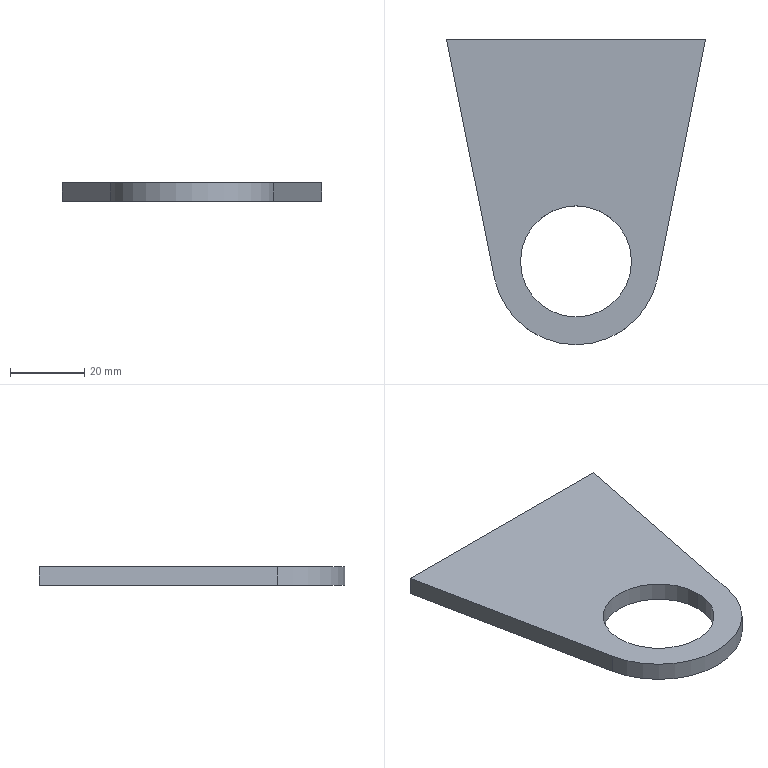Part | STEP file | Spring hanging buckle | 1 solid | 8 faces | box 70 x 82.5 x 5 mm | volume 17833 mm3 | plane 5 | cylinder 3 | commonest cylinder face diameters 30 x2 45 x1
STEP:
#1=CARTESIAN_POINT('',(0.,0.,0.));
#2=DIRECTION('',(0.,0.,1.));
#3=DIRECTION('',(1.,0.,0.));
#4=AXIS2_PLACEMENT_3D('',#1,#2,#3);
#5=CARTESIAN_POINT('',(-15.,0.,2.5));
#6=VERTEX_POINT('',#5);
#7=CARTESIAN_POINT('',(-15.,0.,-2.5));
#8=VERTEX_POINT('',#7);
#9=CARTESIAN_POINT('',(-15.,0.,2.5));
#10=DIRECTION('',(0.,0.,-1.));
#11=VECTOR('',#10,1.);
#12=LINE('',#9,#11);
#13=CARTESIAN_POINT('',(0.,0.,2.5));
#14=DIRECTION('',(0.,0.,-1.));
#15=DIRECTION('',(-1.,0.,0.));
#16=AXIS2_PLACEMENT_3D('',#13,#14,#15);
#17=CYLINDRICAL_SURFACE('',#16,15.);
#18=CARTESIAN_POINT('',(6.283,0.));
#19=DIRECTION('',(0.,1.));
#20=VECTOR('',#19,1.);
#21=LINE('',#18,#20);
#22=(GEOMETRIC_REPRESENTATION_CONTEXT(2)PARAMETRIC_REPRESENTATION_CONTEXT()REPRESENTATION_CONTEXT('',''));
#23=DEFINITIONAL_REPRESENTATION('',(#21),#22);
#24=PCURVE('',#17,#23);
#25=CARTESIAN_POINT('',(0.,0.,2.5));
#26=DIRECTION('',(0.,0.,-1.));
#27=DIRECTION('',(-1.,0.,0.));
#28=AXIS2_PLACEMENT_3D('',#25,#26,#27);
#29=CYLINDRICAL_SURFACE('',#28,15.);
#30=CARTESIAN_POINT('',(0.,0.));
#31=DIRECTION('',(0.,1.));
#32=VECTOR('',#31,1.);
#33=LINE('',#30,#32);
#34=(GEOMETRIC_REPRESENTATION_CONTEXT(2)PARAMETRIC_REPRESENTATION_CONTEXT()REPRESENTATION_CONTEXT('',''));
#35=DEFINITIONAL_REPRESENTATION('',(#33),#34);
#36=PCURVE('',#29,#35);
#37=SURFACE_CURVE('',#12,(#24,#36),.PCURVE_S1.);
#38=EDGE_CURVE('',#6,#8,#37,.T.);
#39=ORIENTED_EDGE('',*,*,#38,.T.);
#40=CARTESIAN_POINT('',(15.,0.,-2.5));
#41=VERTEX_POINT('',#40);
#42=CARTESIAN_POINT('',(0.,0.,-2.5));
#43=DIRECTION('',(0.,0.,1.));
#44=DIRECTION('',(-1.,0.,0.));
#45=AXIS2_PLACEMENT_3D('',#42,#43,#44);
#46=CIRCLE('',#45,15.);
#47=CARTESIAN_POINT('',(6.283,5.));
#48=DIRECTION('',(-1.,0.));
#49=VECTOR('',#48,1.);
#50=LINE('',#47,#49);
#51=(GEOMETRIC_REPRESENTATION_CONTEXT(2)PARAMETRIC_REPRESENTATION_CONTEXT()REPRESENTATION_CONTEXT('',''));
#52=DEFINITIONAL_REPRESENTATION('',(#50),#51);
#53=PCURVE('',#17,#52);
#54=CARTESIAN_POINT('',(0.,0.,-2.5));
#55=DIRECTION('',(0.,0.,1.));
#56=DIRECTION('',(1.,0.,0.));
#57=AXIS2_PLACEMENT_3D('',#54,#55,#56);
#58=PLANE('',#57);
#59=CARTESIAN_POINT('',(0.,0.));
#60=DIRECTION('',(-1.,0.));
#61=AXIS2_PLACEMENT_2D('',#59,#60);
#62=CIRCLE('',#61,15.);
#63=(GEOMETRIC_REPRESENTATION_CONTEXT(2)PARAMETRIC_REPRESENTATION_CONTEXT()REPRESENTATION_CONTEXT('',''));
#64=DEFINITIONAL_REPRESENTATION('',(#62),#63);
#65=PCURVE('',#58,#64);
#66=SURFACE_CURVE('',#46,(#53,#65),.PCURVE_S1.);
#67=EDGE_CURVE('',#8,#41,#66,.T.);
#68=ORIENTED_EDGE('',*,*,#67,.T.);
#69=CARTESIAN_POINT('',(15.,0.,2.5));
#70=VERTEX_POINT('',#69);
#71=CARTESIAN_POINT('',(15.,0.,2.5));
#72=DIRECTION('',(0.,0.,-1.));
#73=VECTOR('',#72,1.);
#74=LINE('',#71,#73);
#75=CARTESIAN_POINT('',(3.142,0.));
#76=DIRECTION('',(0.,1.));
#77=VECTOR('',#76,1.);
#78=LINE('',#75,#77);
#79=(GEOMETRIC_REPRESENTATION_CONTEXT(2)PARAMETRIC_REPRESENTATION_CONTEXT()REPRESENTATION_CONTEXT('',''));
#80=DEFINITIONAL_REPRESENTATION('',(#78),#79);
#81=PCURVE('',#17,#80);
#82=CARTESIAN_POINT('',(3.142,0.));
#83=DIRECTION('',(0.,1.));
#84=VECTOR('',#83,1.);
#85=LINE('',#82,#84);
#86=(GEOMETRIC_REPRESENTATION_CONTEXT(2)PARAMETRIC_REPRESENTATION_CONTEXT()REPRESENTATION_CONTEXT('',''));
#87=DEFINITIONAL_REPRESENTATION('',(#85),#86);
#88=PCURVE('',#29,#87);
#89=SURFACE_CURVE('',#74,(#81,#88),.PCURVE_S1.);
#90=EDGE_CURVE('',#70,#41,#89,.T.);
#91=ORIENTED_EDGE('',*,*,#90,.F.);
#92=CARTESIAN_POINT('',(0.,0.,2.5));
#93=DIRECTION('',(0.,0.,-1.));
#94=DIRECTION('',(-1.,0.,0.));
#95=AXIS2_PLACEMENT_3D('',#92,#93,#94);
#96=CIRCLE('',#95,15.);
#97=CARTESIAN_POINT('',(0.,0.));
#98=DIRECTION('',(1.,0.));
#99=VECTOR('',#98,1.);
#100=LINE('',#97,#99);
#101=(GEOMETRIC_REPRESENTATION_CONTEXT(2)PARAMETRIC_REPRESENTATION_CONTEXT()REPRESENTATION_CONTEXT('',''));
#102=DEFINITIONAL_REPRESENTATION('',(#100),#101);
#103=PCURVE('',#17,#102);
#104=CARTESIAN_POINT('',(0.,0.,2.5));
#105=DIRECTION('',(0.,0.,1.));
#106=DIRECTION('',(1.,0.,0.));
#107=AXIS2_PLACEMENT_3D('',#104,#105,#106);
#108=PLANE('',#107);
#109=CARTESIAN_POINT('',(-15.,0.));
#110=CARTESIAN_POINT('',(-15.,25.981));
#111=CARTESIAN_POINT('',(7.5,12.99));
#112=CARTESIAN_POINT('',(30.,0.));
#113=CARTESIAN_POINT('',(7.5,-12.99));
#114=CARTESIAN_POINT('',(-15.,-25.981));
#115=CARTESIAN_POINT('',(-15.,0.));
#116=(BOUNDED_CURVE()B_SPLINE_CURVE(2,(#109,#110,#111,#112,#113,#114,#115),.UNSPECIFIED.,.T.,.F.)B_SPLINE_CURVE_WITH_KNOTS((1,2,2,2,2,1),(-2.094,0.,2.094,4.189,6.283,8.378),.UNSPECIFIED.)CURVE()GEOMETRIC_REPRESENTATION_ITEM()RATIONAL_B_SPLINE_CURVE((1.,0.5,1.,0.5,1.,0.5,1.))REPRESENTATION_ITEM(''));
#117=(GEOMETRIC_REPRESENTATION_CONTEXT(2)PARAMETRIC_REPRESENTATION_CONTEXT()REPRESENTATION_CONTEXT('',''));
#118=DEFINITIONAL_REPRESENTATION('',(#116),#117);
#119=PCURVE('',#108,#118);
#120=SURFACE_CURVE('',#96,(#103,#119),.PCURVE_S1.);
#121=EDGE_CURVE('',#70,#6,#120,.T.);
#122=ORIENTED_EDGE('',*,*,#121,.T.);
#123=EDGE_LOOP('',(#39,#68,#91,#122));
#124=FACE_BOUND('',#123,.F.);
#125=ADVANCED_FACE('',(#124),#17,.F.);
#126=CARTESIAN_POINT('',(0.,0.,2.5));
#127=DIRECTION('',(0.,0.,-1.));
#128=DIRECTION('',(-1.,0.,0.));
#129=AXIS2_PLACEMENT_3D('',#126,#127,#128);
#130=CIRCLE('',#129,15.);
#131=CARTESIAN_POINT('',(-15.,0.));
#132=CARTESIAN_POINT('',(-15.,25.981));
#133=CARTESIAN_POINT('',(7.5,12.99));
#134=CARTESIAN_POINT('',(30.,0.));
#135=CARTESIAN_POINT('',(7.5,-12.99));
#136=CARTESIAN_POINT('',(-15.,-25.981));
#137=CARTESIAN_POINT('',(-15.,0.));
#138=(BOUNDED_CURVE()B_SPLINE_CURVE(2,(#131,#132,#133,#134,#135,#136,#137),.UNSPECIFIED.,.T.,.F.)B_SPLINE_CURVE_WITH_KNOTS((1,2,2,2,2,1),(-2.094,0.,2.094,4.189,6.283,8.378),.UNSPECIFIED.)CURVE()GEOMETRIC_REPRESENTATION_ITEM()RATIONAL_B_SPLINE_CURVE((1.,0.5,1.,0.5,1.,0.5,1.))REPRESENTATION_ITEM(''));
#139=(GEOMETRIC_REPRESENTATION_CONTEXT(2)PARAMETRIC_REPRESENTATION_CONTEXT()REPRESENTATION_CONTEXT('',''));
#140=DEFINITIONAL_REPRESENTATION('',(#138),#139);
#141=PCURVE('',#108,#140);
#142=CARTESIAN_POINT('',(0.,0.));
#143=DIRECTION('',(1.,0.));
#144=VECTOR('',#143,1.);
#145=LINE('',#142,#144);
#146=(GEOMETRIC_REPRESENTATION_CONTEXT(2)PARAMETRIC_REPRESENTATION_CONTEXT()REPRESENTATION_CONTEXT('',''));
#147=DEFINITIONAL_REPRESENTATION('',(#145),#146);
#148=PCURVE('',#29,#147);
#149=SURFACE_CURVE('',#130,(#141,#148),.PCURVE_S1.);
#150=EDGE_CURVE('',#6,#70,#149,.T.);
#151=ORIENTED_EDGE('',*,*,#150,.T.);
#152=ORIENTED_EDGE('',*,*,#121,.T.);
#153=EDGE_LOOP('',(#151,#152));
#154=FACE_BOUND('',#153,.T.);
#155=CARTESIAN_POINT('',(35.,60.,2.5));
#156=VERTEX_POINT('',#155);
#157=CARTESIAN_POINT('',(-35.,60.,2.5));
#158=VERTEX_POINT('',#157);
#159=CARTESIAN_POINT('',(0.,60.,2.5));
#160=DIRECTION('',(-1.,0.,0.));
#161=VECTOR('',#160,1.);
#162=LINE('',#159,#161);
#163=CARTESIAN_POINT('',(0.,60.));
#164=DIRECTION('',(-1.,0.));
#165=VECTOR('',#164,1.);
#166=LINE('',#163,#165);
#167=(GEOMETRIC_REPRESENTATION_CONTEXT(2)PARAMETRIC_REPRESENTATION_CONTEXT()REPRESENTATION_CONTEXT('',''));
#168=DEFINITIONAL_REPRESENTATION('',(#166),#167);
#169=PCURVE('',#108,#168);
#170=CARTESIAN_POINT('',(35.,60.,2.5));
#171=DIRECTION('',(0.,-1.,0.));
#172=DIRECTION('',(1.,0.,0.));
#173=AXIS2_PLACEMENT_3D('',#170,#171,#172);
#174=PLANE('',#173);
#175=CARTESIAN_POINT('',(-35.,0.));
#176=DIRECTION('',(-1.,0.));
#177=VECTOR('',#176,1.);
#178=LINE('',#175,#177);
#179=(GEOMETRIC_REPRESENTATION_CONTEXT(2)PARAMETRIC_REPRESENTATION_CONTEXT()REPRESENTATION_CONTEXT('',''));
#180=DEFINITIONAL_REPRESENTATION('',(#178),#179);
#181=PCURVE('',#174,#180);
#182=SURFACE_CURVE('',#162,(#169,#181),.PCURVE_S1.);
#183=EDGE_CURVE('',#156,#158,#182,.T.);
#184=ORIENTED_EDGE('',*,*,#183,.T.);
#185=CARTESIAN_POINT('',(-22.059,-4.431,2.5));
#186=VERTEX_POINT('',#185);
#187=CARTESIAN_POINT('',(-35.,60.,2.5));
#188=DIRECTION('',(0.1969,-0.9804,0.));
#189=VECTOR('',#188,1.);
#190=LINE('',#187,#189);
#191=CARTESIAN_POINT('',(-35.,60.));
#192=DIRECTION('',(0.1969,-0.9804));
#193=VECTOR('',#192,1.);
#194=LINE('',#191,#193);
#195=(GEOMETRIC_REPRESENTATION_CONTEXT(2)PARAMETRIC_REPRESENTATION_CONTEXT()REPRESENTATION_CONTEXT('',''));
#196=DEFINITIONAL_REPRESENTATION('',(#194),#195);
#197=PCURVE('',#108,#196);
#198=CARTESIAN_POINT('',(-35.,60.,2.5));
#199=DIRECTION('',(0.9804,0.1969,0.));
#200=DIRECTION('',(-0.1969,0.9804,0.));
#201=AXIS2_PLACEMENT_3D('',#198,#199,#200);
#202=PLANE('',#201);
#203=CARTESIAN_POINT('',(0.,0.));
#204=DIRECTION('',(-1.,0.));
#205=VECTOR('',#204,1.);
#206=LINE('',#203,#205);
#207=(GEOMETRIC_REPRESENTATION_CONTEXT(2)PARAMETRIC_REPRESENTATION_CONTEXT()REPRESENTATION_CONTEXT('',''));
#208=DEFINITIONAL_REPRESENTATION('',(#206),#207);
#209=PCURVE('',#202,#208);
#210=SURFACE_CURVE('',#190,(#197,#209),.PCURVE_S1.);
#211=EDGE_CURVE('',#158,#186,#210,.T.);
#212=ORIENTED_EDGE('',*,*,#211,.T.);
#213=CARTESIAN_POINT('',(22.059,-4.431,2.5));
#214=VERTEX_POINT('',#213);
#215=CARTESIAN_POINT('',(0.,0.,2.5));
#216=DIRECTION('',(0.,0.,1.));
#217=DIRECTION('',(-1.,0.,0.));
#218=AXIS2_PLACEMENT_3D('',#215,#216,#217);
#219=CIRCLE('',#218,22.5);
#220=CARTESIAN_POINT('',(0.,0.));
#221=DIRECTION('',(-1.,0.));
#222=AXIS2_PLACEMENT_2D('',#220,#221);
#223=CIRCLE('',#222,22.5);
#224=(GEOMETRIC_REPRESENTATION_CONTEXT(2)PARAMETRIC_REPRESENTATION_CONTEXT()REPRESENTATION_CONTEXT('',''));
#225=DEFINITIONAL_REPRESENTATION('',(#223),#224);
#226=PCURVE('',#108,#225);
#227=CARTESIAN_POINT('',(0.,0.,2.5));
#228=DIRECTION('',(0.,0.,-1.));
#229=DIRECTION('',(-1.,0.,0.));
#230=AXIS2_PLACEMENT_3D('',#227,#228,#229);
#231=CYLINDRICAL_SURFACE('',#230,22.5);
#232=CARTESIAN_POINT('',(6.283,0.));
#233=DIRECTION('',(-1.,0.));
#234=VECTOR('',#233,1.);
#235=LINE('',#232,#234);
#236=(GEOMETRIC_REPRESENTATION_CONTEXT(2)PARAMETRIC_REPRESENTATION_CONTEXT()REPRESENTATION_CONTEXT('',''));
#237=DEFINITIONAL_REPRESENTATION('',(#235),#236);
#238=PCURVE('',#231,#237);
#239=SURFACE_CURVE('',#219,(#226,#238),.PCURVE_S1.);
#240=EDGE_CURVE('',#186,#214,#239,.T.);
#241=ORIENTED_EDGE('',*,*,#240,.T.);
#242=CARTESIAN_POINT('',(22.059,-4.431,2.5));
#243=DIRECTION('',(0.1969,0.9804,0.));
#244=VECTOR('',#243,1.);
#245=LINE('',#242,#244);
#246=CARTESIAN_POINT('',(22.059,-4.431));
#247=DIRECTION('',(0.1969,0.9804));
#248=VECTOR('',#247,1.);
#249=LINE('',#246,#248);
#250=(GEOMETRIC_REPRESENTATION_CONTEXT(2)PARAMETRIC_REPRESENTATION_CONTEXT()REPRESENTATION_CONTEXT('',''));
#251=DEFINITIONAL_REPRESENTATION('',(#249),#250);
#252=PCURVE('',#108,#251);
#253=CARTESIAN_POINT('',(22.059,-4.431,2.5));
#254=DIRECTION('',(-0.9804,0.1969,0.));
#255=DIRECTION('',(-0.1969,-0.9804,0.));
#256=AXIS2_PLACEMENT_3D('',#253,#254,#255);
#257=PLANE('',#256);
#258=CARTESIAN_POINT('',(0.,0.));
#259=DIRECTION('',(-1.,0.));
#260=VECTOR('',#259,1.);
#261=LINE('',#258,#260);
#262=(GEOMETRIC_REPRESENTATION_CONTEXT(2)PARAMETRIC_REPRESENTATION_CONTEXT()REPRESENTATION_CONTEXT('',''));
#263=DEFINITIONAL_REPRESENTATION('',(#261),#262);
#264=PCURVE('',#257,#263);
#265=SURFACE_CURVE('',#245,(#252,#264),.PCURVE_S1.);
#266=EDGE_CURVE('',#214,#156,#265,.T.);
#267=ORIENTED_EDGE('',*,*,#266,.T.);
#268=EDGE_LOOP('',(#184,#212,#241,#267));
#269=FACE_BOUND('',#268,.T.);
#270=ADVANCED_FACE('',(#154,#269),#108,.T.);
#271=CARTESIAN_POINT('',(0.,0.,-2.5));
#272=DIRECTION('',(0.,0.,1.));
#273=DIRECTION('',(-1.,0.,0.));
#274=AXIS2_PLACEMENT_3D('',#271,#272,#273);
#275=CIRCLE('',#274,15.);
#276=CARTESIAN_POINT('',(6.283,5.));
#277=DIRECTION('',(-1.,0.));
#278=VECTOR('',#277,1.);
#279=LINE('',#276,#278);
#280=(GEOMETRIC_REPRESENTATION_CONTEXT(2)PARAMETRIC_REPRESENTATION_CONTEXT()REPRESENTATION_CONTEXT('',''));
#281=DEFINITIONAL_REPRESENTATION('',(#279),#280);
#282=PCURVE('',#29,#281);
#283=CARTESIAN_POINT('',(0.,0.));
#284=DIRECTION('',(-1.,0.));
#285=AXIS2_PLACEMENT_2D('',#283,#284);
#286=CIRCLE('',#285,15.);
#287=(GEOMETRIC_REPRESENTATION_CONTEXT(2)PARAMETRIC_REPRESENTATION_CONTEXT()REPRESENTATION_CONTEXT('',''));
#288=DEFINITIONAL_REPRESENTATION('',(#286),#287);
#289=PCURVE('',#58,#288);
#290=SURFACE_CURVE('',#275,(#282,#289),.PCURVE_S1.);
#291=EDGE_CURVE('',#41,#8,#290,.T.);
#292=ORIENTED_EDGE('',*,*,#291,.T.);
#293=ORIENTED_EDGE('',*,*,#38,.F.);
#294=ORIENTED_EDGE('',*,*,#150,.T.);
#295=ORIENTED_EDGE('',*,*,#90,.T.);
#296=EDGE_LOOP('',(#292,#293,#294,#295));
#297=FACE_BOUND('',#296,.F.);
#298=ADVANCED_FACE('',(#297),#29,.F.);
#299=CARTESIAN_POINT('',(-22.059,-4.431,-2.5));
#300=VERTEX_POINT('',#299);
#301=CARTESIAN_POINT('',(-22.059,-4.431,2.5));
#302=DIRECTION('',(0.,0.,-1.));
#303=VECTOR('',#302,1.);
#304=LINE('',#301,#303);
#305=CARTESIAN_POINT('',(-65.717,0.));
#306=DIRECTION('',(0.,-1.));
#307=VECTOR('',#306,1.);
#308=LINE('',#305,#307);
#309=(GEOMETRIC_REPRESENTATION_CONTEXT(2)PARAMETRIC_REPRESENTATION_CONTEXT()REPRESENTATION_CONTEXT('',''));
#310=DEFINITIONAL_REPRESENTATION('',(#308),#309);
#311=PCURVE('',#202,#310);
#312=CARTESIAN_POINT('',(6.085,0.));
#313=DIRECTION('',(0.,1.));
#314=VECTOR('',#313,1.);
#315=LINE('',#312,#314);
#316=(GEOMETRIC_REPRESENTATION_CONTEXT(2)PARAMETRIC_REPRESENTATION_CONTEXT()REPRESENTATION_CONTEXT('',''));
#317=DEFINITIONAL_REPRESENTATION('',(#315),#316);
#318=PCURVE('',#231,#317);
#319=SURFACE_CURVE('',#304,(#311,#318),.PCURVE_S1.);
#320=EDGE_CURVE('',#186,#300,#319,.T.);
#321=ORIENTED_EDGE('',*,*,#320,.F.);
#322=ORIENTED_EDGE('',*,*,#211,.F.);
#323=CARTESIAN_POINT('',(-35.,60.,-2.5));
#324=VERTEX_POINT('',#323);
#325=CARTESIAN_POINT('',(-35.,60.,2.5));
#326=DIRECTION('',(0.,0.,1.));
#327=VECTOR('',#326,1.);
#328=LINE('',#325,#327);
#329=CARTESIAN_POINT('',(0.,0.));
#330=DIRECTION('',(0.,1.));
#331=VECTOR('',#330,1.);
#332=LINE('',#329,#331);
#333=(GEOMETRIC_REPRESENTATION_CONTEXT(2)PARAMETRIC_REPRESENTATION_CONTEXT()REPRESENTATION_CONTEXT('',''));
#334=DEFINITIONAL_REPRESENTATION('',(#332),#333);
#335=PCURVE('',#202,#334);
#336=CARTESIAN_POINT('',(-70.,0.));
#337=DIRECTION('',(0.,1.));
#338=VECTOR('',#337,1.);
#339=LINE('',#336,#338);
#340=(GEOMETRIC_REPRESENTATION_CONTEXT(2)PARAMETRIC_REPRESENTATION_CONTEXT()REPRESENTATION_CONTEXT('',''));
#341=DEFINITIONAL_REPRESENTATION('',(#339),#340);
#342=PCURVE('',#174,#341);
#343=SURFACE_CURVE('',#328,(#335,#342),.PCURVE_S1.);
#344=EDGE_CURVE('',#324,#158,#343,.T.);
#345=ORIENTED_EDGE('',*,*,#344,.F.);
#346=CARTESIAN_POINT('',(-35.,60.,-2.5));
#347=DIRECTION('',(-0.1969,0.9804,0.));
#348=VECTOR('',#347,1.);
#349=LINE('',#346,#348);
#350=CARTESIAN_POINT('',(0.,-5.));
#351=DIRECTION('',(1.,0.));
#352=VECTOR('',#351,1.);
#353=LINE('',#350,#352);
#354=(GEOMETRIC_REPRESENTATION_CONTEXT(2)PARAMETRIC_REPRESENTATION_CONTEXT()REPRESENTATION_CONTEXT('',''));
#355=DEFINITIONAL_REPRESENTATION('',(#353),#354);
#356=PCURVE('',#202,#355);
#357=CARTESIAN_POINT('',(-35.,60.));
#358=DIRECTION('',(-0.1969,0.9804));
#359=VECTOR('',#358,1.);
#360=LINE('',#357,#359);
#361=(GEOMETRIC_REPRESENTATION_CONTEXT(2)PARAMETRIC_REPRESENTATION_CONTEXT()REPRESENTATION_CONTEXT('',''));
#362=DEFINITIONAL_REPRESENTATION('',(#360),#361);
#363=PCURVE('',#58,#362);
#364=SURFACE_CURVE('',#349,(#356,#363),.PCURVE_S1.);
#365=EDGE_CURVE('',#300,#324,#364,.T.);
#366=ORIENTED_EDGE('',*,*,#365,.F.);
#367=EDGE_LOOP('',(#321,#322,#345,#366));
#368=FACE_BOUND('',#367,.T.);
#369=ADVANCED_FACE('',(#368),#202,.F.);
#370=ORIENTED_EDGE('',*,*,#344,.T.);
#371=ORIENTED_EDGE('',*,*,#183,.F.);
#372=CARTESIAN_POINT('',(35.,60.,-2.5));
#373=VERTEX_POINT('',#372);
#374=CARTESIAN_POINT('',(35.,60.,2.5));
#375=DIRECTION('',(0.,0.,1.));
#376=VECTOR('',#375,1.);
#377=LINE('',#374,#376);
#378=CARTESIAN_POINT('',(0.,0.));
#379=DIRECTION('',(0.,1.));
#380=VECTOR('',#379,1.);
#381=LINE('',#378,#380);
#382=(GEOMETRIC_REPRESENTATION_CONTEXT(2)PARAMETRIC_REPRESENTATION_CONTEXT()REPRESENTATION_CONTEXT('',''));
#383=DEFINITIONAL_REPRESENTATION('',(#381),#382);
#384=PCURVE('',#174,#383);
#385=CARTESIAN_POINT('',(-65.717,0.));
#386=DIRECTION('',(0.,1.));
#387=VECTOR('',#386,1.);
#388=LINE('',#385,#387);
#389=(GEOMETRIC_REPRESENTATION_CONTEXT(2)PARAMETRIC_REPRESENTATION_CONTEXT()REPRESENTATION_CONTEXT('',''));
#390=DEFINITIONAL_REPRESENTATION('',(#388),#389);
#391=PCURVE('',#257,#390);
#392=SURFACE_CURVE('',#377,(#384,#391),.PCURVE_S1.);
#393=EDGE_CURVE('',#373,#156,#392,.T.);
#394=ORIENTED_EDGE('',*,*,#393,.F.);
#395=CARTESIAN_POINT('',(35.,60.,-2.5));
#396=DIRECTION('',(1.,0.,0.));
#397=VECTOR('',#396,1.);
#398=LINE('',#395,#397);
#399=CARTESIAN_POINT('',(0.,-5.));
#400=DIRECTION('',(1.,0.));
#401=VECTOR('',#400,1.);
#402=LINE('',#399,#401);
#403=(GEOMETRIC_REPRESENTATION_CONTEXT(2)PARAMETRIC_REPRESENTATION_CONTEXT()REPRESENTATION_CONTEXT('',''));
#404=DEFINITIONAL_REPRESENTATION('',(#402),#403);
#405=PCURVE('',#174,#404);
#406=CARTESIAN_POINT('',(35.,60.));
#407=DIRECTION('',(1.,0.));
#408=VECTOR('',#407,1.);
#409=LINE('',#406,#408);
#410=(GEOMETRIC_REPRESENTATION_CONTEXT(2)PARAMETRIC_REPRESENTATION_CONTEXT()REPRESENTATION_CONTEXT('',''));
#411=DEFINITIONAL_REPRESENTATION('',(#409),#410);
#412=PCURVE('',#58,#411);
#413=SURFACE_CURVE('',#398,(#405,#412),.PCURVE_S1.);
#414=EDGE_CURVE('',#324,#373,#413,.T.);
#415=ORIENTED_EDGE('',*,*,#414,.F.);
#416=EDGE_LOOP('',(#370,#371,#394,#415));
#417=FACE_BOUND('',#416,.T.);
#418=ADVANCED_FACE('',(#417),#174,.F.);
#419=ORIENTED_EDGE('',*,*,#393,.T.);
#420=ORIENTED_EDGE('',*,*,#266,.F.);
#421=CARTESIAN_POINT('',(22.059,-4.431,-2.5));
#422=VERTEX_POINT('',#421);
#423=CARTESIAN_POINT('',(22.059,-4.431,2.5));
#424=DIRECTION('',(0.,0.,1.));
#425=VECTOR('',#424,1.);
#426=LINE('',#423,#425);
#427=CARTESIAN_POINT('',(0.,0.));
#428=DIRECTION('',(0.,1.));
#429=VECTOR('',#428,1.);
#430=LINE('',#427,#429);
#431=(GEOMETRIC_REPRESENTATION_CONTEXT(2)PARAMETRIC_REPRESENTATION_CONTEXT()REPRESENTATION_CONTEXT('',''));
#432=DEFINITIONAL_REPRESENTATION('',(#430),#431);
#433=PCURVE('',#257,#432);
#434=CARTESIAN_POINT('',(3.34,0.));
#435=DIRECTION('',(0.,-1.));
#436=VECTOR('',#435,1.);
#437=LINE('',#434,#436);
#438=(GEOMETRIC_REPRESENTATION_CONTEXT(2)PARAMETRIC_REPRESENTATION_CONTEXT()REPRESENTATION_CONTEXT('',''));
#439=DEFINITIONAL_REPRESENTATION('',(#437),#438);
#440=PCURVE('',#231,#439);
#441=SURFACE_CURVE('',#426,(#433,#440),.PCURVE_S1.);
#442=EDGE_CURVE('',#422,#214,#441,.T.);
#443=ORIENTED_EDGE('',*,*,#442,.F.);
#444=CARTESIAN_POINT('',(22.059,-4.431,-2.5));
#445=DIRECTION('',(-0.1969,-0.9804,0.));
#446=VECTOR('',#445,1.);
#447=LINE('',#444,#446);
#448=CARTESIAN_POINT('',(0.,-5.));
#449=DIRECTION('',(1.,0.));
#450=VECTOR('',#449,1.);
#451=LINE('',#448,#450);
#452=(GEOMETRIC_REPRESENTATION_CONTEXT(2)PARAMETRIC_REPRESENTATION_CONTEXT()REPRESENTATION_CONTEXT('',''));
#453=DEFINITIONAL_REPRESENTATION('',(#451),#452);
#454=PCURVE('',#257,#453);
#455=CARTESIAN_POINT('',(22.059,-4.431));
#456=DIRECTION('',(-0.1969,-0.9804));
#457=VECTOR('',#456,1.);
#458=LINE('',#455,#457);
#459=(GEOMETRIC_REPRESENTATION_CONTEXT(2)PARAMETRIC_REPRESENTATION_CONTEXT()REPRESENTATION_CONTEXT('',''));
#460=DEFINITIONAL_REPRESENTATION('',(#458),#459);
#461=PCURVE('',#58,#460);
#462=SURFACE_CURVE('',#447,(#454,#461),.PCURVE_S1.);
#463=EDGE_CURVE('',#373,#422,#462,.T.);
#464=ORIENTED_EDGE('',*,*,#463,.F.);
#465=EDGE_LOOP('',(#419,#420,#443,#464));
#466=FACE_BOUND('',#465,.T.);
#467=ADVANCED_FACE('',(#466),#257,.F.);
#468=ORIENTED_EDGE('',*,*,#240,.F.);
#469=ORIENTED_EDGE('',*,*,#320,.T.);
#470=CARTESIAN_POINT('',(0.,0.,-2.5));
#471=DIRECTION('',(0.,0.,1.));
#472=DIRECTION('',(-1.,0.,0.));
#473=AXIS2_PLACEMENT_3D('',#470,#471,#472);
#474=CIRCLE('',#473,22.5);
#475=CARTESIAN_POINT('',(6.283,5.));
#476=DIRECTION('',(-1.,0.));
#477=VECTOR('',#476,1.);
#478=LINE('',#475,#477);
#479=(GEOMETRIC_REPRESENTATION_CONTEXT(2)PARAMETRIC_REPRESENTATION_CONTEXT()REPRESENTATION_CONTEXT('',''));
#480=DEFINITIONAL_REPRESENTATION('',(#478),#479);
#481=PCURVE('',#231,#480);
#482=CARTESIAN_POINT('',(0.,0.));
#483=DIRECTION('',(-1.,0.));
#484=AXIS2_PLACEMENT_2D('',#482,#483);
#485=CIRCLE('',#484,22.5);
#486=(GEOMETRIC_REPRESENTATION_CONTEXT(2)PARAMETRIC_REPRESENTATION_CONTEXT()REPRESENTATION_CONTEXT('',''));
#487=DEFINITIONAL_REPRESENTATION('',(#485),#486);
#488=PCURVE('',#58,#487);
#489=SURFACE_CURVE('',#474,(#481,#488),.PCURVE_S1.);
#490=EDGE_CURVE('',#300,#422,#489,.T.);
#491=ORIENTED_EDGE('',*,*,#490,.T.);
#492=ORIENTED_EDGE('',*,*,#442,.T.);
#493=EDGE_LOOP('',(#468,#469,#491,#492));
#494=FACE_BOUND('',#493,.T.);
#495=ADVANCED_FACE('',(#494),#231,.T.);
#496=ORIENTED_EDGE('',*,*,#67,.T.);
#497=ORIENTED_EDGE('',*,*,#291,.T.);
#498=EDGE_LOOP('',(#496,#497));
#499=FACE_BOUND('',#498,.T.);
#500=ORIENTED_EDGE('',*,*,#365,.T.);
#501=ORIENTED_EDGE('',*,*,#414,.T.);
#502=ORIENTED_EDGE('',*,*,#463,.T.);
#503=ORIENTED_EDGE('',*,*,#490,.F.);
#504=EDGE_LOOP('',(#500,#501,#502,#503));
#505=FACE_BOUND('',#504,.T.);
#506=ADVANCED_FACE('',(#499,#505),#58,.F.);
#507=CLOSED_SHELL('',(#125,#270,#298,#369,#418,#467,#495,#506));
#508=MANIFOLD_SOLID_BREP('',#507);
#509=(LENGTH_UNIT()NAMED_UNIT(*)SI_UNIT(.MILLI.,.METRE.));
#510=UNCERTAINTY_MEASURE_WITH_UNIT(LENGTH_MEASURE(0.0000001),#509,'','');
#511=(NAMED_UNIT(*)PLANE_ANGLE_UNIT()SI_UNIT($,.RADIAN.));
#512=(NAMED_UNIT(*)SI_UNIT($,.STERADIAN.)SOLID_ANGLE_UNIT());
#513=(GEOMETRIC_REPRESENTATION_CONTEXT(3)GLOBAL_UNCERTAINTY_ASSIGNED_CONTEXT((#510))GLOBAL_UNIT_ASSIGNED_CONTEXT((#509,#511,#512))REPRESENTATION_CONTEXT('',''));
#514=ADVANCED_BREP_SHAPE_REPRESENTATION('',(#4,#508),#513);